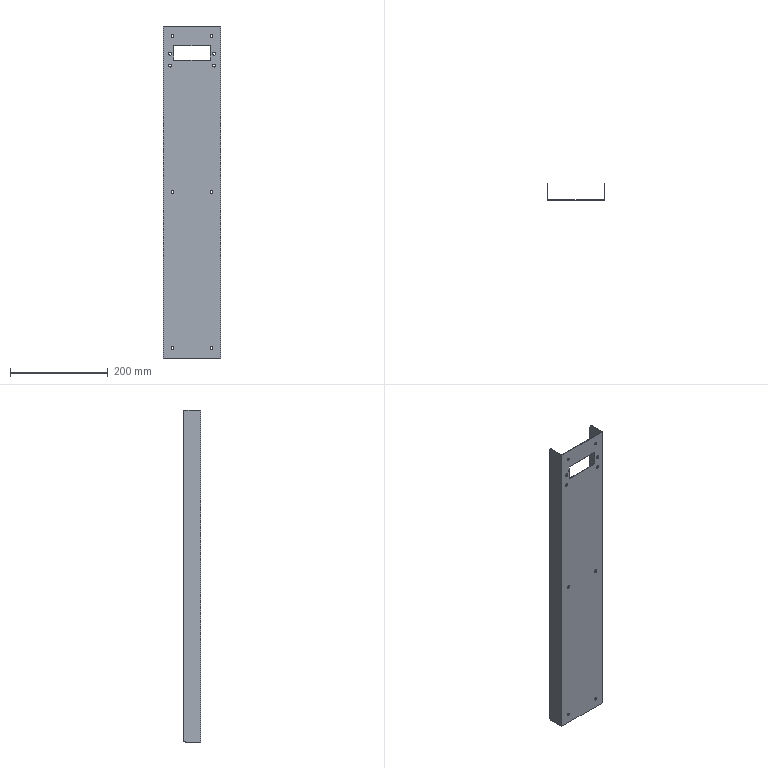Part | STEP file | Cable Carrier Channel | 1 solid | 38 faces | box 118 x 35 x 680 mm | volume 123926 mm3 | cylinder 24 | plane 14 | commonest cylinder face diameters 6 x20 10 x4